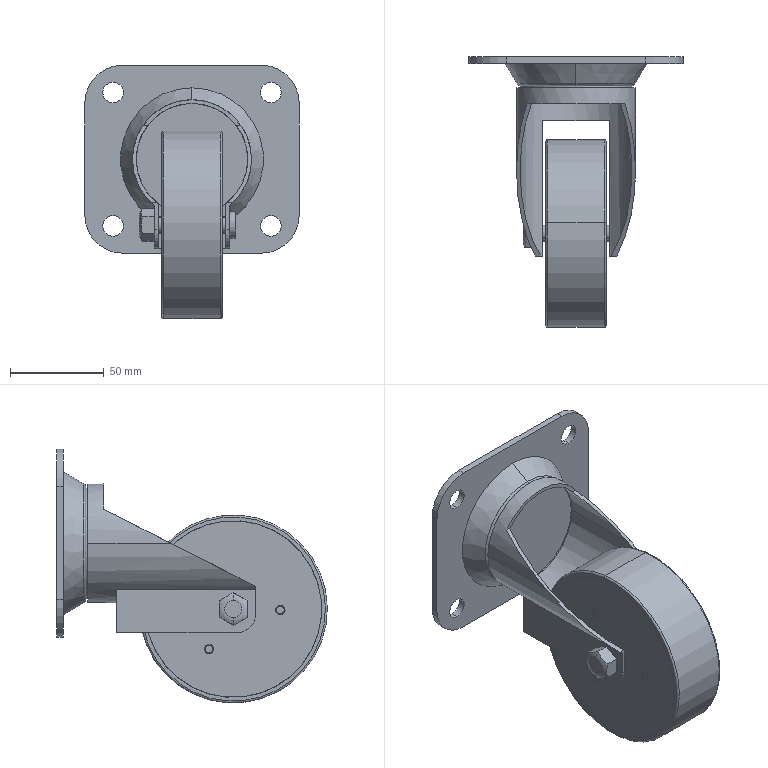Part | SolidWorks | features CompositeCurve 1 | 15 solids | 384 faces | box 114 x 144 x 135 mm | volume 347724 mm3 | torus 132 | cylinder 104 | sphere 68 | plane 62 | cone 18 | commonest cylinder face diameters 5 x24 11 x8 23 x8 29 x8 35 x8 17 x6